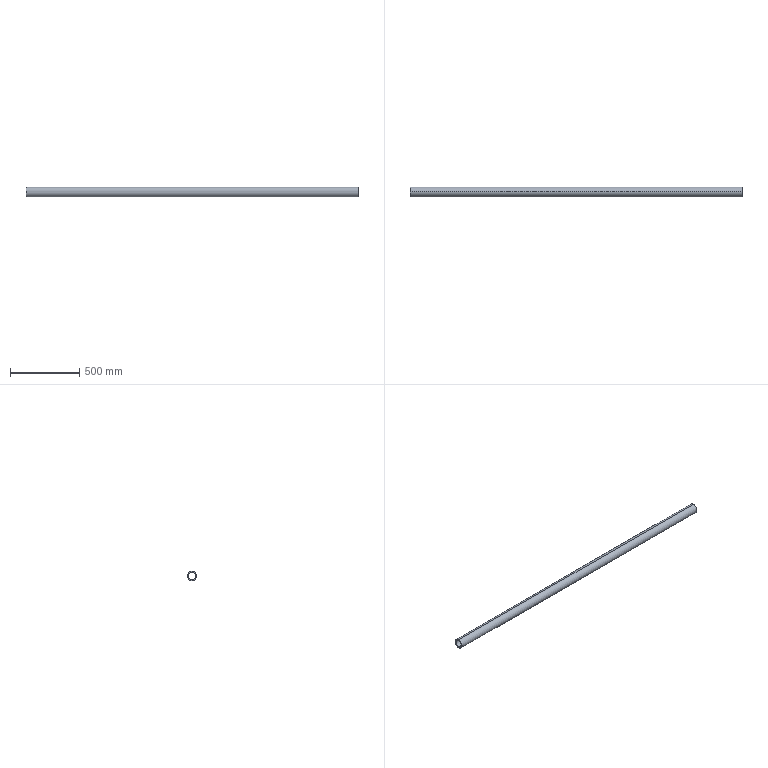Part | STEP file | 1 solid | 6 faces | box 2404 x 70 x 70 mm | volume 3745985 mm3 | cylinder 4 | plane 2 | commonest cylinder face diameters 54 x2 70 x2
STEP:
#1=CARTESIAN_POINT('',(0.,0.,0.));
#2=DIRECTION('',(0.,0.,1.));
#3=DIRECTION('',(1.,0.,0.));
#4=AXIS2_PLACEMENT_3D('',#1,#2,#3);
#5=CARTESIAN_POINT('',(1202.,0.,-35.));
#6=VERTEX_POINT('',#5);
#7=CARTESIAN_POINT('',(1202.,0.,35.));
#8=VERTEX_POINT('',#7);
#9=CARTESIAN_POINT('',(1202.,0.,0.));
#10=DIRECTION('',(1.,0.,0.));
#11=DIRECTION('',(0.,0.,-1.));
#12=AXIS2_PLACEMENT_3D('',#9,#10,#11);
#13=CIRCLE('',#12,35.);
#14=CARTESIAN_POINT('',(1202.,0.,0.));
#15=DIRECTION('',(-1.,0.,0.));
#16=DIRECTION('',(0.,0.,1.));
#17=AXIS2_PLACEMENT_3D('',#14,#15,#16);
#18=CYLINDRICAL_SURFACE('',#17,35.);
#19=CARTESIAN_POINT('',(3.142,0.));
#20=DIRECTION('',(-1.,0.));
#21=VECTOR('',#20,1.);
#22=LINE('',#19,#21);
#23=(GEOMETRIC_REPRESENTATION_CONTEXT(2)PARAMETRIC_REPRESENTATION_CONTEXT()REPRESENTATION_CONTEXT('',''));
#24=DEFINITIONAL_REPRESENTATION('',(#22),#23);
#25=PCURVE('',#18,#24);
#26=CARTESIAN_POINT('',(1202.,0.,0.));
#27=DIRECTION('',(1.,0.,0.));
#28=DIRECTION('',(0.,0.,-1.));
#29=AXIS2_PLACEMENT_3D('',#26,#27,#28);
#30=PLANE('',#29);
#31=CARTESIAN_POINT('',(0.,0.));
#32=DIRECTION('',(1.,0.));
#33=AXIS2_PLACEMENT_2D('',#31,#32);
#34=CIRCLE('',#33,35.);
#35=(GEOMETRIC_REPRESENTATION_CONTEXT(2)PARAMETRIC_REPRESENTATION_CONTEXT()REPRESENTATION_CONTEXT('',''));
#36=DEFINITIONAL_REPRESENTATION('',(#34),#35);
#37=PCURVE('',#30,#36);
#38=SURFACE_CURVE('',#13,(#25,#37),.PCURVE_S1.);
#39=EDGE_CURVE('',#6,#8,#38,.T.);
#40=ORIENTED_EDGE('',*,*,#39,.F.);
#41=CARTESIAN_POINT('',(-1202.,0.,-35.));
#42=VERTEX_POINT('',#41);
#43=CARTESIAN_POINT('',(1202.,0.,-35.));
#44=DIRECTION('',(-1.,0.,0.));
#45=VECTOR('',#44,1.);
#46=LINE('',#43,#45);
#47=CARTESIAN_POINT('',(3.142,0.));
#48=DIRECTION('',(0.,1.));
#49=VECTOR('',#48,1.);
#50=LINE('',#47,#49);
#51=(GEOMETRIC_REPRESENTATION_CONTEXT(2)PARAMETRIC_REPRESENTATION_CONTEXT()REPRESENTATION_CONTEXT('',''));
#52=DEFINITIONAL_REPRESENTATION('',(#50),#51);
#53=PCURVE('',#18,#52);
#54=CARTESIAN_POINT('',(1202.,0.,0.));
#55=DIRECTION('',(-1.,0.,0.));
#56=DIRECTION('',(0.,0.,1.));
#57=AXIS2_PLACEMENT_3D('',#54,#55,#56);
#58=CYLINDRICAL_SURFACE('',#57,35.);
#59=CARTESIAN_POINT('',(3.142,0.));
#60=DIRECTION('',(0.,1.));
#61=VECTOR('',#60,1.);
#62=LINE('',#59,#61);
#63=(GEOMETRIC_REPRESENTATION_CONTEXT(2)PARAMETRIC_REPRESENTATION_CONTEXT()REPRESENTATION_CONTEXT('',''));
#64=DEFINITIONAL_REPRESENTATION('',(#62),#63);
#65=PCURVE('',#58,#64);
#66=SURFACE_CURVE('',#46,(#53,#65),.PCURVE_S1.);
#67=EDGE_CURVE('',#6,#42,#66,.T.);
#68=ORIENTED_EDGE('',*,*,#67,.T.);
#69=CARTESIAN_POINT('',(-1202.,0.,35.));
#70=VERTEX_POINT('',#69);
#71=CARTESIAN_POINT('',(-1202.,0.,0.));
#72=DIRECTION('',(1.,0.,0.));
#73=DIRECTION('',(0.,0.,-1.));
#74=AXIS2_PLACEMENT_3D('',#71,#72,#73);
#75=CIRCLE('',#74,35.);
#76=CARTESIAN_POINT('',(3.142,2404.));
#77=DIRECTION('',(-1.,0.));
#78=VECTOR('',#77,1.);
#79=LINE('',#76,#78);
#80=(GEOMETRIC_REPRESENTATION_CONTEXT(2)PARAMETRIC_REPRESENTATION_CONTEXT()REPRESENTATION_CONTEXT('',''));
#81=DEFINITIONAL_REPRESENTATION('',(#79),#80);
#82=PCURVE('',#18,#81);
#83=CARTESIAN_POINT('',(-1202.,0.,0.));
#84=DIRECTION('',(1.,0.,0.));
#85=DIRECTION('',(0.,0.,-1.));
#86=AXIS2_PLACEMENT_3D('',#83,#84,#85);
#87=PLANE('',#86);
#88=CARTESIAN_POINT('',(0.,0.));
#89=DIRECTION('',(1.,0.));
#90=AXIS2_PLACEMENT_2D('',#88,#89);
#91=CIRCLE('',#90,35.);
#92=(GEOMETRIC_REPRESENTATION_CONTEXT(2)PARAMETRIC_REPRESENTATION_CONTEXT()REPRESENTATION_CONTEXT('',''));
#93=DEFINITIONAL_REPRESENTATION('',(#91),#92);
#94=PCURVE('',#87,#93);
#95=SURFACE_CURVE('',#75,(#82,#94),.PCURVE_S1.);
#96=EDGE_CURVE('',#42,#70,#95,.T.);
#97=ORIENTED_EDGE('',*,*,#96,.T.);
#98=CARTESIAN_POINT('',(1202.,0.,35.));
#99=DIRECTION('',(-1.,0.,0.));
#100=VECTOR('',#99,1.);
#101=LINE('',#98,#100);
#102=CARTESIAN_POINT('',(0.,0.));
#103=DIRECTION('',(0.,1.));
#104=VECTOR('',#103,1.);
#105=LINE('',#102,#104);
#106=(GEOMETRIC_REPRESENTATION_CONTEXT(2)PARAMETRIC_REPRESENTATION_CONTEXT()REPRESENTATION_CONTEXT('',''));
#107=DEFINITIONAL_REPRESENTATION('',(#105),#106);
#108=PCURVE('',#18,#107);
#109=CARTESIAN_POINT('',(6.283,0.));
#110=DIRECTION('',(0.,1.));
#111=VECTOR('',#110,1.);
#112=LINE('',#109,#111);
#113=(GEOMETRIC_REPRESENTATION_CONTEXT(2)PARAMETRIC_REPRESENTATION_CONTEXT()REPRESENTATION_CONTEXT('',''));
#114=DEFINITIONAL_REPRESENTATION('',(#112),#113);
#115=PCURVE('',#58,#114);
#116=SURFACE_CURVE('',#101,(#108,#115),.PCURVE_S1.);
#117=EDGE_CURVE('',#8,#70,#116,.T.);
#118=ORIENTED_EDGE('',*,*,#117,.F.);
#119=EDGE_LOOP('',(#40,#68,#97,#118));
#120=FACE_BOUND('',#119,.T.);
#121=ADVANCED_FACE('',(#120),#18,.T.);
#122=CARTESIAN_POINT('',(1202.,0.,27.));
#123=VERTEX_POINT('',#122);
#124=CARTESIAN_POINT('',(-1202.,0.,27.));
#125=VERTEX_POINT('',#124);
#126=CARTESIAN_POINT('',(1202.,0.,27.));
#127=DIRECTION('',(-1.,0.,0.));
#128=VECTOR('',#127,1.);
#129=LINE('',#126,#128);
#130=CARTESIAN_POINT('',(1202.,0.,0.));
#131=DIRECTION('',(-1.,0.,0.));
#132=DIRECTION('',(0.,0.,1.));
#133=AXIS2_PLACEMENT_3D('',#130,#131,#132);
#134=CYLINDRICAL_SURFACE('',#133,27.);
#135=CARTESIAN_POINT('',(6.283,0.));
#136=DIRECTION('',(0.,1.));
#137=VECTOR('',#136,1.);
#138=LINE('',#135,#137);
#139=(GEOMETRIC_REPRESENTATION_CONTEXT(2)PARAMETRIC_REPRESENTATION_CONTEXT()REPRESENTATION_CONTEXT('',''));
#140=DEFINITIONAL_REPRESENTATION('',(#138),#139);
#141=PCURVE('',#134,#140);
#142=CARTESIAN_POINT('',(1202.,0.,0.));
#143=DIRECTION('',(-1.,0.,0.));
#144=DIRECTION('',(0.,0.,1.));
#145=AXIS2_PLACEMENT_3D('',#142,#143,#144);
#146=CYLINDRICAL_SURFACE('',#145,27.);
#147=CARTESIAN_POINT('',(0.,0.));
#148=DIRECTION('',(0.,1.));
#149=VECTOR('',#148,1.);
#150=LINE('',#147,#149);
#151=(GEOMETRIC_REPRESENTATION_CONTEXT(2)PARAMETRIC_REPRESENTATION_CONTEXT()REPRESENTATION_CONTEXT('',''));
#152=DEFINITIONAL_REPRESENTATION('',(#150),#151);
#153=PCURVE('',#146,#152);
#154=SURFACE_CURVE('',#129,(#141,#153),.PCURVE_S1.);
#155=EDGE_CURVE('',#123,#125,#154,.T.);
#156=ORIENTED_EDGE('',*,*,#155,.T.);
#157=CARTESIAN_POINT('',(-1202.,0.,-27.));
#158=VERTEX_POINT('',#157);
#159=CARTESIAN_POINT('',(-1202.,0.,0.));
#160=DIRECTION('',(1.,0.,0.));
#161=DIRECTION('',(0.,0.,-1.));
#162=AXIS2_PLACEMENT_3D('',#159,#160,#161);
#163=CIRCLE('',#162,27.);
#164=CARTESIAN_POINT('',(9.425,2404.));
#165=DIRECTION('',(-1.,0.));
#166=VECTOR('',#165,1.);
#167=LINE('',#164,#166);
#168=(GEOMETRIC_REPRESENTATION_CONTEXT(2)PARAMETRIC_REPRESENTATION_CONTEXT()REPRESENTATION_CONTEXT('',''));
#169=DEFINITIONAL_REPRESENTATION('',(#167),#168);
#170=PCURVE('',#134,#169);
#171=CARTESIAN_POINT('',(0.,0.));
#172=DIRECTION('',(1.,0.));
#173=AXIS2_PLACEMENT_2D('',#171,#172);
#174=CIRCLE('',#173,27.);
#175=(GEOMETRIC_REPRESENTATION_CONTEXT(2)PARAMETRIC_REPRESENTATION_CONTEXT()REPRESENTATION_CONTEXT('',''));
#176=DEFINITIONAL_REPRESENTATION('',(#174),#175);
#177=PCURVE('',#87,#176);
#178=SURFACE_CURVE('',#163,(#170,#177),.PCURVE_S1.);
#179=EDGE_CURVE('',#125,#158,#178,.T.);
#180=ORIENTED_EDGE('',*,*,#179,.T.);
#181=CARTESIAN_POINT('',(1202.,0.,-27.));
#182=VERTEX_POINT('',#181);
#183=CARTESIAN_POINT('',(1202.,0.,-27.));
#184=DIRECTION('',(-1.,0.,0.));
#185=VECTOR('',#184,1.);
#186=LINE('',#183,#185);
#187=CARTESIAN_POINT('',(3.142,0.));
#188=DIRECTION('',(0.,1.));
#189=VECTOR('',#188,1.);
#190=LINE('',#187,#189);
#191=(GEOMETRIC_REPRESENTATION_CONTEXT(2)PARAMETRIC_REPRESENTATION_CONTEXT()REPRESENTATION_CONTEXT('',''));
#192=DEFINITIONAL_REPRESENTATION('',(#190),#191);
#193=PCURVE('',#134,#192);
#194=CARTESIAN_POINT('',(3.142,0.));
#195=DIRECTION('',(0.,1.));
#196=VECTOR('',#195,1.);
#197=LINE('',#194,#196);
#198=(GEOMETRIC_REPRESENTATION_CONTEXT(2)PARAMETRIC_REPRESENTATION_CONTEXT()REPRESENTATION_CONTEXT('',''));
#199=DEFINITIONAL_REPRESENTATION('',(#197),#198);
#200=PCURVE('',#146,#199);
#201=SURFACE_CURVE('',#186,(#193,#200),.PCURVE_S1.);
#202=EDGE_CURVE('',#182,#158,#201,.T.);
#203=ORIENTED_EDGE('',*,*,#202,.F.);
#204=CARTESIAN_POINT('',(1202.,0.,0.));
#205=DIRECTION('',(1.,0.,0.));
#206=DIRECTION('',(0.,0.,-1.));
#207=AXIS2_PLACEMENT_3D('',#204,#205,#206);
#208=CIRCLE('',#207,27.);
#209=CARTESIAN_POINT('',(9.425,0.));
#210=DIRECTION('',(-1.,0.));
#211=VECTOR('',#210,1.);
#212=LINE('',#209,#211);
#213=(GEOMETRIC_REPRESENTATION_CONTEXT(2)PARAMETRIC_REPRESENTATION_CONTEXT()REPRESENTATION_CONTEXT('',''));
#214=DEFINITIONAL_REPRESENTATION('',(#212),#213);
#215=PCURVE('',#134,#214);
#216=CARTESIAN_POINT('',(0.,0.));
#217=DIRECTION('',(1.,0.));
#218=AXIS2_PLACEMENT_2D('',#216,#217);
#219=CIRCLE('',#218,27.);
#220=(GEOMETRIC_REPRESENTATION_CONTEXT(2)PARAMETRIC_REPRESENTATION_CONTEXT()REPRESENTATION_CONTEXT('',''));
#221=DEFINITIONAL_REPRESENTATION('',(#219),#220);
#222=PCURVE('',#30,#221);
#223=SURFACE_CURVE('',#208,(#215,#222),.PCURVE_S1.);
#224=EDGE_CURVE('',#123,#182,#223,.T.);
#225=ORIENTED_EDGE('',*,*,#224,.F.);
#226=EDGE_LOOP('',(#156,#180,#203,#225));
#227=FACE_BOUND('',#226,.F.);
#228=ADVANCED_FACE('',(#227),#134,.F.);
#229=CARTESIAN_POINT('',(-1202.,0.,0.));
#230=DIRECTION('',(1.,0.,0.));
#231=DIRECTION('',(0.,0.,-1.));
#232=AXIS2_PLACEMENT_3D('',#229,#230,#231);
#233=CIRCLE('',#232,27.);
#234=CARTESIAN_POINT('',(3.142,2404.));
#235=DIRECTION('',(-1.,0.));
#236=VECTOR('',#235,1.);
#237=LINE('',#234,#236);
#238=(GEOMETRIC_REPRESENTATION_CONTEXT(2)PARAMETRIC_REPRESENTATION_CONTEXT()REPRESENTATION_CONTEXT('',''));
#239=DEFINITIONAL_REPRESENTATION('',(#237),#238);
#240=PCURVE('',#146,#239);
#241=CARTESIAN_POINT('',(0.,0.));
#242=DIRECTION('',(1.,0.));
#243=AXIS2_PLACEMENT_2D('',#241,#242);
#244=CIRCLE('',#243,27.);
#245=(GEOMETRIC_REPRESENTATION_CONTEXT(2)PARAMETRIC_REPRESENTATION_CONTEXT()REPRESENTATION_CONTEXT('',''));
#246=DEFINITIONAL_REPRESENTATION('',(#244),#245);
#247=PCURVE('',#87,#246);
#248=SURFACE_CURVE('',#233,(#240,#247),.PCURVE_S1.);
#249=EDGE_CURVE('',#158,#125,#248,.T.);
#250=ORIENTED_EDGE('',*,*,#249,.T.);
#251=ORIENTED_EDGE('',*,*,#155,.F.);
#252=CARTESIAN_POINT('',(1202.,0.,0.));
#253=DIRECTION('',(1.,0.,0.));
#254=DIRECTION('',(0.,0.,-1.));
#255=AXIS2_PLACEMENT_3D('',#252,#253,#254);
#256=CIRCLE('',#255,27.);
#257=CARTESIAN_POINT('',(3.142,0.));
#258=DIRECTION('',(-1.,0.));
#259=VECTOR('',#258,1.);
#260=LINE('',#257,#259);
#261=(GEOMETRIC_REPRESENTATION_CONTEXT(2)PARAMETRIC_REPRESENTATION_CONTEXT()REPRESENTATION_CONTEXT('',''));
#262=DEFINITIONAL_REPRESENTATION('',(#260),#261);
#263=PCURVE('',#146,#262);
#264=CARTESIAN_POINT('',(0.,0.));
#265=DIRECTION('',(1.,0.));
#266=AXIS2_PLACEMENT_2D('',#264,#265);
#267=CIRCLE('',#266,27.);
#268=(GEOMETRIC_REPRESENTATION_CONTEXT(2)PARAMETRIC_REPRESENTATION_CONTEXT()REPRESENTATION_CONTEXT('',''));
#269=DEFINITIONAL_REPRESENTATION('',(#267),#268);
#270=PCURVE('',#30,#269);
#271=SURFACE_CURVE('',#256,(#263,#270),.PCURVE_S1.);
#272=EDGE_CURVE('',#182,#123,#271,.T.);
#273=ORIENTED_EDGE('',*,*,#272,.F.);
#274=ORIENTED_EDGE('',*,*,#202,.T.);
#275=EDGE_LOOP('',(#250,#251,#273,#274));
#276=FACE_BOUND('',#275,.F.);
#277=ADVANCED_FACE('',(#276),#146,.F.);
#278=ORIENTED_EDGE('',*,*,#67,.F.);
#279=CARTESIAN_POINT('',(1202.,0.,0.));
#280=DIRECTION('',(1.,0.,0.));
#281=DIRECTION('',(0.,0.,-1.));
#282=AXIS2_PLACEMENT_3D('',#279,#280,#281);
#283=CIRCLE('',#282,35.);
#284=CARTESIAN_POINT('',(9.425,0.));
#285=DIRECTION('',(-1.,0.));
#286=VECTOR('',#285,1.);
#287=LINE('',#284,#286);
#288=(GEOMETRIC_REPRESENTATION_CONTEXT(2)PARAMETRIC_REPRESENTATION_CONTEXT()REPRESENTATION_CONTEXT('',''));
#289=DEFINITIONAL_REPRESENTATION('',(#287),#288);
#290=PCURVE('',#58,#289);
#291=CARTESIAN_POINT('',(0.,0.));
#292=DIRECTION('',(1.,0.));
#293=AXIS2_PLACEMENT_2D('',#291,#292);
#294=CIRCLE('',#293,35.);
#295=(GEOMETRIC_REPRESENTATION_CONTEXT(2)PARAMETRIC_REPRESENTATION_CONTEXT()REPRESENTATION_CONTEXT('',''));
#296=DEFINITIONAL_REPRESENTATION('',(#294),#295);
#297=PCURVE('',#30,#296);
#298=SURFACE_CURVE('',#283,(#290,#297),.PCURVE_S1.);
#299=EDGE_CURVE('',#8,#6,#298,.T.);
#300=ORIENTED_EDGE('',*,*,#299,.F.);
#301=ORIENTED_EDGE('',*,*,#117,.T.);
#302=CARTESIAN_POINT('',(-1202.,0.,0.));
#303=DIRECTION('',(1.,0.,0.));
#304=DIRECTION('',(0.,0.,-1.));
#305=AXIS2_PLACEMENT_3D('',#302,#303,#304);
#306=CIRCLE('',#305,35.);
#307=CARTESIAN_POINT('',(9.425,2404.));
#308=DIRECTION('',(-1.,0.));
#309=VECTOR('',#308,1.);
#310=LINE('',#307,#309);
#311=(GEOMETRIC_REPRESENTATION_CONTEXT(2)PARAMETRIC_REPRESENTATION_CONTEXT()REPRESENTATION_CONTEXT('',''));
#312=DEFINITIONAL_REPRESENTATION('',(#310),#311);
#313=PCURVE('',#58,#312);
#314=CARTESIAN_POINT('',(0.,0.));
#315=DIRECTION('',(1.,0.));
#316=AXIS2_PLACEMENT_2D('',#314,#315);
#317=CIRCLE('',#316,35.);
#318=(GEOMETRIC_REPRESENTATION_CONTEXT(2)PARAMETRIC_REPRESENTATION_CONTEXT()REPRESENTATION_CONTEXT('',''));
#319=DEFINITIONAL_REPRESENTATION('',(#317),#318);
#320=PCURVE('',#87,#319);
#321=SURFACE_CURVE('',#306,(#313,#320),.PCURVE_S1.);
#322=EDGE_CURVE('',#70,#42,#321,.T.);
#323=ORIENTED_EDGE('',*,*,#322,.T.);
#324=EDGE_LOOP('',(#278,#300,#301,#323));
#325=FACE_BOUND('',#324,.T.);
#326=ADVANCED_FACE('',(#325),#58,.T.);
#327=ORIENTED_EDGE('',*,*,#224,.F.);
#328=ORIENTED_EDGE('',*,*,#272,.F.);
#329=EDGE_LOOP('',(#327,#328));
#330=FACE_BOUND('',#329,.T.);
#331=ORIENTED_EDGE('',*,*,#299,.T.);
#332=ORIENTED_EDGE('',*,*,#39,.T.);
#333=EDGE_LOOP('',(#331,#332));
#334=FACE_BOUND('',#333,.T.);
#335=ADVANCED_FACE('',(#330,#334),#30,.T.);
#336=ORIENTED_EDGE('',*,*,#179,.T.);
#337=ORIENTED_EDGE('',*,*,#249,.T.);
#338=EDGE_LOOP('',(#336,#337));
#339=FACE_BOUND('',#338,.T.);
#340=ORIENTED_EDGE('',*,*,#322,.F.);
#341=ORIENTED_EDGE('',*,*,#96,.F.);
#342=EDGE_LOOP('',(#340,#341));
#343=FACE_BOUND('',#342,.T.);
#344=ADVANCED_FACE('',(#339,#343),#87,.F.);
#345=CLOSED_SHELL('',(#121,#228,#277,#326,#335,#344));
#346=MANIFOLD_SOLID_BREP('',#345);
#347=(LENGTH_UNIT()NAMED_UNIT(*)SI_UNIT(.MILLI.,.METRE.));
#348=UNCERTAINTY_MEASURE_WITH_UNIT(LENGTH_MEASURE(0.0000001),#347,'','');
#349=(NAMED_UNIT(*)PLANE_ANGLE_UNIT()SI_UNIT($,.RADIAN.));
#350=(NAMED_UNIT(*)SI_UNIT($,.STERADIAN.)SOLID_ANGLE_UNIT());
#351=(GEOMETRIC_REPRESENTATION_CONTEXT(3)GLOBAL_UNCERTAINTY_ASSIGNED_CONTEXT((#348))GLOBAL_UNIT_ASSIGNED_CONTEXT((#347,#349,#350))REPRESENTATION_CONTEXT('',''));
#352=ADVANCED_BREP_SHAPE_REPRESENTATION('',(#4,#346),#351);